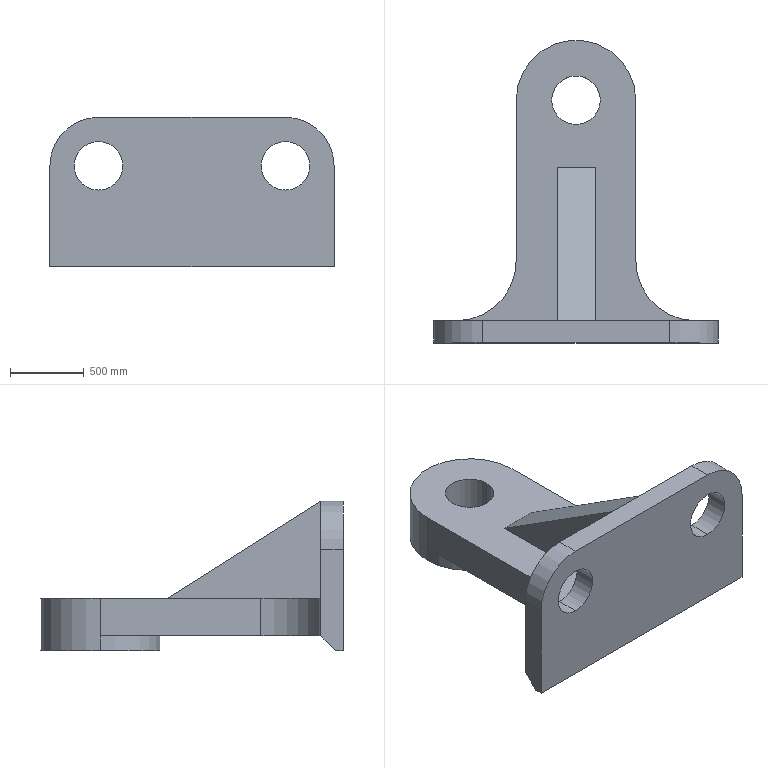Part | SolidWorks | features ICE 4, Chamfer 1, Extrusion 1, Fillet 1 | 1 solid | 28 faces | box 1930 x 2057 x 1016 mm | volume 760890020 mm3 | plane 16 | cylinder 12 | commonest cylinder face diameters 330.2 x6 812.8 x4 660.4 x2
STEP:
#1=CARTESIAN_POINT('',(6.5,65.,-6.));
#2=VERTEX_POINT('',#1);
#3=CARTESIAN_POINT('',(-6.5,65.,-6.));
#4=VERTEX_POINT('',#3);
#5=CARTESIAN_POINT('',(0.,65.,-6.));
#6=DIRECTION('',(0.,0.,-1.));
#7=DIRECTION('',(-1.,0.,0.));
#8=AXIS2_PLACEMENT_3D('',#5,#6,#7);
#9=CIRCLE('',#8,6.5);
#10=EDGE_CURVE('',#2,#4,#9,.T.);
#11=ORIENTED_EDGE('',*,*,#10,.F.);
#12=CARTESIAN_POINT('',(6.5,65.,-20.));
#13=VERTEX_POINT('',#12);
#14=CARTESIAN_POINT('',(6.5,65.,-6.));
#15=DIRECTION('',(0.,0.,-1.));
#16=VECTOR('',#15,39.37);
#17=LINE('',#14,#16);
#18=EDGE_CURVE('',#2,#13,#17,.T.);
#19=ORIENTED_EDGE('',*,*,#18,.T.);
#20=CARTESIAN_POINT('',(-6.5,65.,-20.));
#21=VERTEX_POINT('',#20);
#22=CARTESIAN_POINT('',(0.,65.,-20.));
#23=DIRECTION('',(0.,0.,-1.));
#24=DIRECTION('',(-1.,0.,0.));
#25=AXIS2_PLACEMENT_3D('',#22,#23,#24);
#26=CIRCLE('',#25,6.5);
#27=EDGE_CURVE('',#13,#21,#26,.T.);
#28=ORIENTED_EDGE('',*,*,#27,.T.);
#29=CARTESIAN_POINT('',(-6.5,65.,-6.));
#30=DIRECTION('',(0.,0.,-1.));
#31=VECTOR('',#30,39.37);
#32=LINE('',#29,#31);
#33=EDGE_CURVE('',#4,#21,#32,.T.);
#34=ORIENTED_EDGE('',*,*,#33,.F.);
#35=EDGE_LOOP('',(#11,#19,#28,#34));
#36=FACE_OUTER_BOUND('',#35,.T.);
#37=CARTESIAN_POINT('',(0.,65.,-6.));
#38=DIRECTION('',(0.,0.,-1.));
#39=DIRECTION('',(-1.,0.,0.));
#40=AXIS2_PLACEMENT_3D('',#37,#38,#39);
#41=CYLINDRICAL_SURFACE('',#40,6.5);
#42=ADVANCED_FACE('',(#36),#41,.F.);
#43=CARTESIAN_POINT('',(16.,65.,-6.));
#44=VERTEX_POINT('',#43);
#45=CARTESIAN_POINT('',(16.,65.,-16.));
#46=VERTEX_POINT('',#45);
#47=CARTESIAN_POINT('',(16.,65.,-6.));
#48=DIRECTION('',(0.,0.,-1.));
#49=VECTOR('',#48,39.37);
#50=LINE('',#47,#49);
#51=EDGE_CURVE('',#44,#46,#50,.T.);
#52=ORIENTED_EDGE('',*,*,#51,.T.);
#53=CARTESIAN_POINT('',(16.,65.,-20.));
#54=VERTEX_POINT('',#53);
#55=CARTESIAN_POINT('',(16.,65.,-6.));
#56=DIRECTION('',(0.,0.,-1.));
#57=VECTOR('',#56,39.37);
#58=LINE('',#55,#57);
#59=EDGE_CURVE('',#46,#54,#58,.T.);
#60=ORIENTED_EDGE('',*,*,#59,.T.);
#61=CARTESIAN_POINT('',(-16.,65.,-20.));
#62=VERTEX_POINT('',#61);
#63=CARTESIAN_POINT('',(0.,65.,-20.));
#64=DIRECTION('',(0.,0.,-1.));
#65=DIRECTION('',(-1.,0.,0.));
#66=AXIS2_PLACEMENT_3D('',#63,#64,#65);
#67=CIRCLE('',#66,16.);
#68=EDGE_CURVE('',#62,#54,#67,.T.);
#69=ORIENTED_EDGE('',*,*,#68,.F.);
#70=CARTESIAN_POINT('',(-16.,65.,-16.));
#71=VERTEX_POINT('',#70);
#72=CARTESIAN_POINT('',(-16.,65.,-6.));
#73=DIRECTION('',(0.,0.,-1.));
#74=VECTOR('',#73,39.37);
#75=LINE('',#72,#74);
#76=EDGE_CURVE('',#71,#62,#75,.T.);
#77=ORIENTED_EDGE('',*,*,#76,.F.);
#78=CARTESIAN_POINT('',(-16.,65.,-6.));
#79=VERTEX_POINT('',#78);
#80=CARTESIAN_POINT('',(-16.,65.,-6.));
#81=DIRECTION('',(0.,0.,-1.));
#82=VECTOR('',#81,39.37);
#83=LINE('',#80,#82);
#84=EDGE_CURVE('',#79,#71,#83,.T.);
#85=ORIENTED_EDGE('',*,*,#84,.F.);
#86=CARTESIAN_POINT('',(0.,65.,-6.));
#87=DIRECTION('',(0.,0.,-1.));
#88=DIRECTION('',(-1.,0.,0.));
#89=AXIS2_PLACEMENT_3D('',#86,#87,#88);
#90=CIRCLE('',#89,16.);
#91=EDGE_CURVE('',#79,#44,#90,.T.);
#92=ORIENTED_EDGE('',*,*,#91,.T.);
#93=EDGE_LOOP('',(#52,#60,#69,#77,#85,#92));
#94=FACE_OUTER_BOUND('',#93,.T.);
#95=CARTESIAN_POINT('',(0.,65.,-6.));
#96=DIRECTION('',(0.,0.,-1.));
#97=DIRECTION('',(-1.,0.,0.));
#98=AXIS2_PLACEMENT_3D('',#95,#96,#97);
#99=CYLINDRICAL_SURFACE('',#98,16.);
#100=ADVANCED_FACE('',(#94),#99,.T.);
#101=CARTESIAN_POINT('',(25.,6.,0.5));
#102=VERTEX_POINT('',#101);
#103=CARTESIAN_POINT('',(25.,6.,13.5));
#104=VERTEX_POINT('',#103);
#105=CARTESIAN_POINT('',(25.,6.,7.));
#106=DIRECTION('',(0.,1.,0.));
#107=DIRECTION('',(0.,0.,1.));
#108=AXIS2_PLACEMENT_3D('',#105,#106,#107);
#109=CIRCLE('',#108,6.5);
#110=EDGE_CURVE('',#102,#104,#109,.T.);
#111=ORIENTED_EDGE('',*,*,#110,.T.);
#112=CARTESIAN_POINT('',(25.,0.,13.5));
#113=VERTEX_POINT('',#112);
#114=CARTESIAN_POINT('',(25.,6.,13.5));
#115=DIRECTION('',(0.,-1.,0.));
#116=VECTOR('',#115,39.37);
#117=LINE('',#114,#116);
#118=EDGE_CURVE('',#104,#113,#117,.T.);
#119=ORIENTED_EDGE('',*,*,#118,.T.);
#120=CARTESIAN_POINT('',(25.,0.,0.5));
#121=VERTEX_POINT('',#120);
#122=CARTESIAN_POINT('',(25.,0.,7.));
#123=DIRECTION('',(0.,1.,0.));
#124=DIRECTION('',(0.,0.,1.));
#125=AXIS2_PLACEMENT_3D('',#122,#123,#124);
#126=CIRCLE('',#125,6.5);
#127=EDGE_CURVE('',#121,#113,#126,.T.);
#128=ORIENTED_EDGE('',*,*,#127,.F.);
#129=CARTESIAN_POINT('',(25.,6.,0.5));
#130=DIRECTION('',(0.,-1.,0.));
#131=VECTOR('',#130,39.37);
#132=LINE('',#129,#131);
#133=EDGE_CURVE('',#102,#121,#132,.T.);
#134=ORIENTED_EDGE('',*,*,#133,.F.);
#135=EDGE_LOOP('',(#111,#119,#128,#134));
#136=FACE_OUTER_BOUND('',#135,.T.);
#137=CARTESIAN_POINT('',(25.,6.,7.));
#138=DIRECTION('',(0.,-1.,0.));
#139=DIRECTION('',(0.,0.,-1.));
#140=AXIS2_PLACEMENT_3D('',#137,#138,#139);
#141=CYLINDRICAL_SURFACE('',#140,6.5);
#142=ADVANCED_FACE('',(#136),#141,.F.);
#143=CARTESIAN_POINT('',(-25.,6.,0.5));
#144=VERTEX_POINT('',#143);
#145=CARTESIAN_POINT('',(-25.,6.,13.5));
#146=VERTEX_POINT('',#145);
#147=CARTESIAN_POINT('',(-25.,6.,7.));
#148=DIRECTION('',(0.,1.,0.));
#149=DIRECTION('',(0.,0.,1.));
#150=AXIS2_PLACEMENT_3D('',#147,#148,#149);
#151=CIRCLE('',#150,6.5);
#152=EDGE_CURVE('',#144,#146,#151,.T.);
#153=ORIENTED_EDGE('',*,*,#152,.T.);
#154=CARTESIAN_POINT('',(-25.,0.,13.5));
#155=VERTEX_POINT('',#154);
#156=CARTESIAN_POINT('',(-25.,6.,13.5));
#157=DIRECTION('',(0.,-1.,0.));
#158=VECTOR('',#157,39.37);
#159=LINE('',#156,#158);
#160=EDGE_CURVE('',#146,#155,#159,.T.);
#161=ORIENTED_EDGE('',*,*,#160,.T.);
#162=CARTESIAN_POINT('',(-25.,0.,0.5));
#163=VERTEX_POINT('',#162);
#164=CARTESIAN_POINT('',(-25.,0.,7.));
#165=DIRECTION('',(0.,1.,0.));
#166=DIRECTION('',(0.,0.,1.));
#167=AXIS2_PLACEMENT_3D('',#164,#165,#166);
#168=CIRCLE('',#167,6.5);
#169=EDGE_CURVE('',#163,#155,#168,.T.);
#170=ORIENTED_EDGE('',*,*,#169,.F.);
#171=CARTESIAN_POINT('',(-25.,6.,0.5));
#172=DIRECTION('',(0.,-1.,0.));
#173=VECTOR('',#172,39.37);
#174=LINE('',#171,#173);
#175=EDGE_CURVE('',#144,#163,#174,.T.);
#176=ORIENTED_EDGE('',*,*,#175,.F.);
#177=EDGE_LOOP('',(#153,#161,#170,#176));
#178=FACE_OUTER_BOUND('',#177,.T.);
#179=CARTESIAN_POINT('',(-25.,6.,7.));
#180=DIRECTION('',(0.,-1.,0.));
#181=DIRECTION('',(0.,0.,-1.));
#182=AXIS2_PLACEMENT_3D('',#179,#180,#181);
#183=CYLINDRICAL_SURFACE('',#182,6.5);
#184=ADVANCED_FACE('',(#178),#183,.F.);
#185=ORIENTED_EDGE('',*,*,#110,.F.);
#186=CARTESIAN_POINT('',(25.,6.,7.));
#187=DIRECTION('',(0.,1.,0.));
#188=DIRECTION('',(0.,0.,1.));
#189=AXIS2_PLACEMENT_3D('',#186,#187,#188);
#190=CIRCLE('',#189,6.5);
#191=EDGE_CURVE('',#104,#102,#190,.T.);
#192=ORIENTED_EDGE('',*,*,#191,.F.);
#193=EDGE_LOOP('',(#185,#192));
#194=FACE_BOUND('',#193,.T.);
#195=CARTESIAN_POINT('',(38.,6.,7.));
#196=VERTEX_POINT('',#195);
#197=CARTESIAN_POINT('',(38.,6.,-16.));
#198=VERTEX_POINT('',#197);
#199=CARTESIAN_POINT('',(38.,6.,7.));
#200=DIRECTION('',(0.,0.,-1.));
#201=VECTOR('',#200,39.37);
#202=LINE('',#199,#201);
#203=EDGE_CURVE('',#196,#198,#202,.T.);
#204=ORIENTED_EDGE('',*,*,#203,.T.);
#205=CARTESIAN_POINT('',(32.,6.,-16.));
#206=VERTEX_POINT('',#205);
#207=CARTESIAN_POINT('',(-38.,6.,-16.));
#208=DIRECTION('',(-1.,0.,0.));
#209=VECTOR('',#208,39.37);
#210=LINE('',#207,#209);
#211=EDGE_CURVE('',#198,#206,#210,.T.);
#212=ORIENTED_EDGE('',*,*,#211,.T.);
#213=CARTESIAN_POINT('',(32.,6.,-6.));
#214=VERTEX_POINT('',#213);
#215=CARTESIAN_POINT('',(32.,6.,-6.));
#216=DIRECTION('',(0.,0.,1.));
#217=VECTOR('',#216,39.37);
#218=LINE('',#215,#217);
#219=EDGE_CURVE('',#206,#214,#218,.T.);
#220=ORIENTED_EDGE('',*,*,#219,.T.);
#221=CARTESIAN_POINT('',(5.262,6.,-6.));
#222=VERTEX_POINT('',#221);
#223=CARTESIAN_POINT('',(0.,6.,-6.));
#224=DIRECTION('',(1.,0.,0.));
#225=VECTOR('',#224,39.37);
#226=LINE('',#223,#225);
#227=EDGE_CURVE('',#222,#214,#226,.T.);
#228=ORIENTED_EDGE('',*,*,#227,.F.);
#229=CARTESIAN_POINT('',(5.262,6.,20.));
#230=VERTEX_POINT('',#229);
#231=CARTESIAN_POINT('',(5.262,6.,-6.));
#232=DIRECTION('',(0.,0.,-1.));
#233=VECTOR('',#232,39.37);
#234=LINE('',#231,#233);
#235=EDGE_CURVE('',#230,#222,#234,.T.);
#236=ORIENTED_EDGE('',*,*,#235,.F.);
#237=CARTESIAN_POINT('',(25.,6.,20.));
#238=VERTEX_POINT('',#237);
#239=CARTESIAN_POINT('',(25.,6.,20.));
#240=DIRECTION('',(1.,0.,0.));
#241=VECTOR('',#240,39.37);
#242=LINE('',#239,#241);
#243=EDGE_CURVE('',#230,#238,#242,.T.);
#244=ORIENTED_EDGE('',*,*,#243,.T.);
#245=CARTESIAN_POINT('',(25.,6.,7.));
#246=DIRECTION('',(0.,1.,0.));
#247=DIRECTION('',(0.,0.,1.));
#248=AXIS2_PLACEMENT_3D('',#245,#246,#247);
#249=CIRCLE('',#248,13.);
#250=EDGE_CURVE('',#238,#196,#249,.T.);
#251=ORIENTED_EDGE('',*,*,#250,.T.);
#252=EDGE_LOOP('',(#204,#212,#220,#228,#236,#244,#251));
#253=FACE_OUTER_BOUND('',#252,.T.);
#254=CARTESIAN_POINT('',(25.,6.,7.));
#255=DIRECTION('',(0.,1.,0.));
#256=DIRECTION('',(0.,0.,1.));
#257=AXIS2_PLACEMENT_3D('',#254,#255,#256);
#258=PLANE('',#257);
#259=ADVANCED_FACE('',(#194,#253),#258,.T.);
#260=ORIENTED_EDGE('',*,*,#152,.F.);
#261=CARTESIAN_POINT('',(-25.,6.,7.));
#262=DIRECTION('',(0.,1.,0.));
#263=DIRECTION('',(0.,0.,1.));
#264=AXIS2_PLACEMENT_3D('',#261,#262,#263);
#265=CIRCLE('',#264,6.5);
#266=EDGE_CURVE('',#146,#144,#265,.T.);
#267=ORIENTED_EDGE('',*,*,#266,.F.);
#268=EDGE_LOOP('',(#260,#267));
#269=FACE_BOUND('',#268,.T.);
#270=CARTESIAN_POINT('',(-32.,6.,-6.));
#271=VERTEX_POINT('',#270);
#272=CARTESIAN_POINT('',(-32.,6.,-16.));
#273=VERTEX_POINT('',#272);
#274=CARTESIAN_POINT('',(-32.,6.,7.));
#275=DIRECTION('',(0.,0.,-1.));
#276=VECTOR('',#275,39.37);
#277=LINE('',#274,#276);
#278=EDGE_CURVE('',#271,#273,#277,.T.);
#279=ORIENTED_EDGE('',*,*,#278,.T.);
#280=CARTESIAN_POINT('',(-38.,6.,-16.));
#281=VERTEX_POINT('',#280);
#282=CARTESIAN_POINT('',(-38.,6.,-16.));
#283=DIRECTION('',(-1.,0.,0.));
#284=VECTOR('',#283,39.37);
#285=LINE('',#282,#284);
#286=EDGE_CURVE('',#273,#281,#285,.T.);
#287=ORIENTED_EDGE('',*,*,#286,.T.);
#288=CARTESIAN_POINT('',(-38.,6.,7.));
#289=VERTEX_POINT('',#288);
#290=CARTESIAN_POINT('',(-38.,6.,7.));
#291=DIRECTION('',(0.,0.,1.));
#292=VECTOR('',#291,39.37);
#293=LINE('',#290,#292);
#294=EDGE_CURVE('',#281,#289,#293,.T.);
#295=ORIENTED_EDGE('',*,*,#294,.T.);
#296=CARTESIAN_POINT('',(-25.,6.,20.));
#297=VERTEX_POINT('',#296);
#298=CARTESIAN_POINT('',(-25.,6.,7.));
#299=DIRECTION('',(0.,1.,0.));
#300=DIRECTION('',(0.,0.,-1.));
#301=AXIS2_PLACEMENT_3D('',#298,#299,#300);
#302=CIRCLE('',#301,13.);
#303=EDGE_CURVE('',#289,#297,#302,.T.);
#304=ORIENTED_EDGE('',*,*,#303,.T.);
#305=CARTESIAN_POINT('',(-5.,6.,20.));
#306=VERTEX_POINT('',#305);
#307=CARTESIAN_POINT('',(25.,6.,20.));
#308=DIRECTION('',(1.,0.,0.));
#309=VECTOR('',#308,39.37);
#310=LINE('',#307,#309);
#311=EDGE_CURVE('',#297,#306,#310,.T.);
#312=ORIENTED_EDGE('',*,*,#311,.T.);
#313=CARTESIAN_POINT('',(-5.,6.,-6.));
#314=VERTEX_POINT('',#313);
#315=CARTESIAN_POINT('',(-5.,6.,-6.));
#316=DIRECTION('',(0.,0.,1.));
#317=VECTOR('',#316,39.37);
#318=LINE('',#315,#317);
#319=EDGE_CURVE('',#314,#306,#318,.T.);
#320=ORIENTED_EDGE('',*,*,#319,.F.);
#321=CARTESIAN_POINT('',(0.,6.,-6.));
#322=DIRECTION('',(1.,0.,0.));
#323=VECTOR('',#322,39.37);
#324=LINE('',#321,#323);
#325=EDGE_CURVE('',#271,#314,#324,.T.);
#326=ORIENTED_EDGE('',*,*,#325,.F.);
#327=EDGE_LOOP('',(#279,#287,#295,#304,#312,#320,#326));
#328=FACE_OUTER_BOUND('',#327,.T.);
#329=CARTESIAN_POINT('',(25.,6.,7.));
#330=DIRECTION('',(0.,1.,0.));
#331=DIRECTION('',(0.,0.,1.));
#332=AXIS2_PLACEMENT_3D('',#329,#330,#331);
#333=PLANE('',#332);
#334=ADVANCED_FACE('',(#269,#328),#333,.T.);
#335=CARTESIAN_POINT('',(-5.,47.,-6.));
#336=VERTEX_POINT('',#335);
#337=CARTESIAN_POINT('',(-5.,47.,-6.));
#338=DIRECTION('',(0.,-1.,0.));
#339=VECTOR('',#338,39.37);
#340=LINE('',#337,#339);
#341=EDGE_CURVE('',#336,#314,#340,.T.);
#342=ORIENTED_EDGE('',*,*,#341,.F.);
#343=CARTESIAN_POINT('',(5.262,47.,-6.));
#344=VERTEX_POINT('',#343);
#345=CARTESIAN_POINT('',(-5.,47.,-6.));
#346=DIRECTION('',(-1.,0.,0.));
#347=VECTOR('',#346,39.37);
#348=LINE('',#345,#347);
#349=EDGE_CURVE('',#344,#336,#348,.T.);
#350=ORIENTED_EDGE('',*,*,#349,.F.);
#351=CARTESIAN_POINT('',(5.262,47.,-6.));
#352=DIRECTION('',(0.,-1.,0.));
#353=VECTOR('',#352,39.37);
#354=LINE('',#351,#353);
#355=EDGE_CURVE('',#344,#222,#354,.T.);
#356=ORIENTED_EDGE('',*,*,#355,.T.);
#357=ORIENTED_EDGE('',*,*,#227,.T.);
#358=CARTESIAN_POINT('',(16.,22.,-6.));
#359=VERTEX_POINT('',#358);
#360=CARTESIAN_POINT('',(32.,22.,-6.));
#361=DIRECTION('',(0.,0.,-1.));
#362=DIRECTION('',(-1.,0.,0.));
#363=AXIS2_PLACEMENT_3D('',#360,#361,#362);
#364=CIRCLE('',#363,16.);
#365=EDGE_CURVE('',#214,#359,#364,.T.);
#366=ORIENTED_EDGE('',*,*,#365,.T.);
#367=CARTESIAN_POINT('',(16.,0.,-6.));
#368=DIRECTION('',(0.,-1.,0.));
#369=VECTOR('',#368,39.37);
#370=LINE('',#367,#369);
#371=EDGE_CURVE('',#44,#359,#370,.T.);
#372=ORIENTED_EDGE('',*,*,#371,.F.);
#373=ORIENTED_EDGE('',*,*,#91,.F.);
#374=CARTESIAN_POINT('',(-16.,22.,-6.));
#375=VERTEX_POINT('',#374);
#376=CARTESIAN_POINT('',(-16.,0.,-6.));
#377=DIRECTION('',(0.,-1.,0.));
#378=VECTOR('',#377,39.37);
#379=LINE('',#376,#378);
#380=EDGE_CURVE('',#79,#375,#379,.T.);
#381=ORIENTED_EDGE('',*,*,#380,.T.);
#382=CARTESIAN_POINT('',(-32.,22.,-6.));
#383=DIRECTION('',(0.,0.,-1.));
#384=DIRECTION('',(-1.,0.,0.));
#385=AXIS2_PLACEMENT_3D('',#382,#383,#384);
#386=CIRCLE('',#385,16.);
#387=EDGE_CURVE('',#375,#271,#386,.T.);
#388=ORIENTED_EDGE('',*,*,#387,.T.);
#389=ORIENTED_EDGE('',*,*,#325,.T.);
#390=EDGE_LOOP('',(#342,#350,#356,#357,#366,#372,#373,#381,#388,#389));
#391=FACE_OUTER_BOUND('',#390,.T.);
#392=CARTESIAN_POINT('',(0.,65.,-6.));
#393=DIRECTION('',(0.,0.,-1.));
#394=DIRECTION('',(-1.,0.,0.));
#395=AXIS2_PLACEMENT_3D('',#392,#393,#394);
#396=CIRCLE('',#395,6.5);
#397=EDGE_CURVE('',#4,#2,#396,.T.);
#398=ORIENTED_EDGE('',*,*,#397,.T.);
#399=ORIENTED_EDGE('',*,*,#10,.T.);
#400=EDGE_LOOP('',(#398,#399));
#401=FACE_BOUND('',#400,.T.);
#402=CARTESIAN_POINT('',(0.,0.,-6.));
#403=DIRECTION('',(0.,0.,-1.));
#404=DIRECTION('',(-1.,0.,0.));
#405=AXIS2_PLACEMENT_3D('',#402,#403,#404);
#406=PLANE('',#405);
#407=ADVANCED_FACE('',(#391,#401),#406,.F.);
#408=CARTESIAN_POINT('',(-16.,22.,-16.));
#409=VERTEX_POINT('',#408);
#410=CARTESIAN_POINT('',(-16.,0.,-16.));
#411=DIRECTION('',(0.,-1.,0.));
#412=VECTOR('',#411,39.37);
#413=LINE('',#410,#412);
#414=EDGE_CURVE('',#71,#409,#413,.T.);
#415=ORIENTED_EDGE('',*,*,#414,.F.);
#416=CARTESIAN_POINT('',(0.,65.,-16.));
#417=DIRECTION('',(0.,0.,1.));
#418=DIRECTION('',(-1.,0.,0.));
#419=AXIS2_PLACEMENT_3D('',#416,#417,#418);
#420=CIRCLE('',#419,16.);
#421=EDGE_CURVE('',#71,#46,#420,.T.);
#422=ORIENTED_EDGE('',*,*,#421,.T.);
#423=CARTESIAN_POINT('',(16.,22.,-16.));
#424=VERTEX_POINT('',#423);
#425=CARTESIAN_POINT('',(16.,0.,-16.));
#426=DIRECTION('',(0.,-1.,0.));
#427=VECTOR('',#426,39.37);
#428=LINE('',#425,#427);
#429=EDGE_CURVE('',#46,#424,#428,.T.);
#430=ORIENTED_EDGE('',*,*,#429,.T.);
#431=CARTESIAN_POINT('',(32.,22.,-16.));
#432=DIRECTION('',(0.,0.,1.));
#433=DIRECTION('',(-1.,0.,0.));
#434=AXIS2_PLACEMENT_3D('',#431,#432,#433);
#435=CIRCLE('',#434,16.);
#436=EDGE_CURVE('',#424,#206,#435,.T.);
#437=ORIENTED_EDGE('',*,*,#436,.T.);
#438=CARTESIAN_POINT('',(0.,6.,-16.));
#439=DIRECTION('',(1.,0.,0.));
#440=VECTOR('',#439,39.37);
#441=LINE('',#438,#440);
#442=EDGE_CURVE('',#273,#206,#441,.T.);
#443=ORIENTED_EDGE('',*,*,#442,.F.);
#444=CARTESIAN_POINT('',(-32.,22.,-16.));
#445=DIRECTION('',(0.,0.,1.));
#446=DIRECTION('',(-1.,0.,0.));
#447=AXIS2_PLACEMENT_3D('',#444,#445,#446);
#448=CIRCLE('',#447,16.);
#449=EDGE_CURVE('',#273,#409,#448,.T.);
#450=ORIENTED_EDGE('',*,*,#449,.T.);
#451=EDGE_LOOP('',(#415,#422,#430,#437,#443,#450));
#452=FACE_OUTER_BOUND('',#451,.T.);
#453=CARTESIAN_POINT('',(0.,0.,-16.));
#454=DIRECTION('',(0.,0.,-1.));
#455=DIRECTION('',(-1.,0.,0.));
#456=AXIS2_PLACEMENT_3D('',#453,#454,#455);
#457=PLANE('',#456);
#458=ADVANCED_FACE('',(#452),#457,.T.);
#459=CARTESIAN_POINT('',(-38.,0.,-20.));
#460=VERTEX_POINT('',#459);
#461=CARTESIAN_POINT('',(-38.,0.,7.));
#462=VERTEX_POINT('',#461);
#463=CARTESIAN_POINT('',(-38.,0.,7.));
#464=DIRECTION('',(0.,0.,1.));
#465=VECTOR('',#464,39.37);
#466=LINE('',#463,#465);
#467=EDGE_CURVE('',#460,#462,#466,.T.);
#468=ORIENTED_EDGE('',*,*,#467,.F.);
#469=CARTESIAN_POINT('',(38.,0.,-20.));
#470=VERTEX_POINT('',#469);
#471=CARTESIAN_POINT('',(38.,0.,-20.));
#472=DIRECTION('',(-1.,0.,0.));
#473=VECTOR('',#472,39.37);
#474=LINE('',#471,#473);
#475=EDGE_CURVE('',#470,#460,#474,.T.);
#476=ORIENTED_EDGE('',*,*,#475,.F.);
#477=CARTESIAN_POINT('',(38.,0.,7.));
#478=VERTEX_POINT('',#477);
#479=CARTESIAN_POINT('',(38.,0.,7.));
#480=DIRECTION('',(0.,0.,-1.));
#481=VECTOR('',#480,39.37);
#482=LINE('',#479,#481);
#483=EDGE_CURVE('',#478,#470,#482,.T.);
#484=ORIENTED_EDGE('',*,*,#483,.F.);
#485=CARTESIAN_POINT('',(25.,0.,20.));
#486=VERTEX_POINT('',#485);
#487=CARTESIAN_POINT('',(25.,0.,7.));
#488=DIRECTION('',(0.,1.,0.));
#489=DIRECTION('',(0.,0.,1.));
#490=AXIS2_PLACEMENT_3D('',#487,#488,#489);
#491=CIRCLE('',#490,13.);
#492=EDGE_CURVE('',#486,#478,#491,.T.);
#493=ORIENTED_EDGE('',*,*,#492,.F.);
#494=CARTESIAN_POINT('',(-25.,0.,20.));
#495=VERTEX_POINT('',#494);
#496=CARTESIAN_POINT('',(25.,0.,20.));
#497=DIRECTION('',(1.,0.,0.));
#498=VECTOR('',#497,39.37);
#499=LINE('',#496,#498);
#500=EDGE_CURVE('',#495,#486,#499,.T.);
#501=ORIENTED_EDGE('',*,*,#500,.F.);
#502=CARTESIAN_POINT('',(-25.,0.,7.));
#503=DIRECTION('',(0.,1.,0.));
#504=DIRECTION('',(0.,0.,-1.));
#505=AXIS2_PLACEMENT_3D('',#502,#503,#504);
#506=CIRCLE('',#505,13.);
#507=EDGE_CURVE('',#462,#495,#506,.T.);
#508=ORIENTED_EDGE('',*,*,#507,.F.);
#509=EDGE_LOOP('',(#468,#476,#484,#493,#501,#508));
#510=FACE_OUTER_BOUND('',#509,.T.);
#511=ORIENTED_EDGE('',*,*,#169,.T.);
#512=CARTESIAN_POINT('',(-25.,0.,7.));
#513=DIRECTION('',(0.,1.,0.));
#514=DIRECTION('',(0.,0.,1.));
#515=AXIS2_PLACEMENT_3D('',#512,#513,#514);
#516=CIRCLE('',#515,6.5);
#517=EDGE_CURVE('',#155,#163,#516,.T.);
#518=ORIENTED_EDGE('',*,*,#517,.T.);
#519=EDGE_LOOP('',(#511,#518));
#520=FACE_BOUND('',#519,.T.);
#521=ORIENTED_EDGE('',*,*,#127,.T.);
#522=CARTESIAN_POINT('',(25.,0.,7.));
#523=DIRECTION('',(0.,1.,0.));
#524=DIRECTION('',(0.,0.,1.));
#525=AXIS2_PLACEMENT_3D('',#522,#523,#524);
#526=CIRCLE('',#525,6.5);
#527=EDGE_CURVE('',#113,#121,#526,.T.);
#528=ORIENTED_EDGE('',*,*,#527,.T.);
#529=EDGE_LOOP('',(#521,#528));
#530=FACE_BOUND('',#529,.T.);
#531=CARTESIAN_POINT('',(25.,0.,7.));
#532=DIRECTION('',(0.,1.,0.));
#533=DIRECTION('',(0.,0.,1.));
#534=AXIS2_PLACEMENT_3D('',#531,#532,#533);
#535=PLANE('',#534);
#536=ADVANCED_FACE('',(#510,#520,#530),#535,.F.);
#537=ORIENTED_EDGE('',*,*,#294,.F.);
#538=CARTESIAN_POINT('',(-38.,2.,-20.));
#539=VERTEX_POINT('',#538);
#540=CARTESIAN_POINT('',(-38.,6.,-16.));
#541=DIRECTION('',(0.,-0.7071,-0.7071));
#542=VECTOR('',#541,39.37);
#543=LINE('',#540,#542);
#544=EDGE_CURVE('',#281,#539,#543,.T.);
#545=ORIENTED_EDGE('',*,*,#544,.T.);
#546=CARTESIAN_POINT('',(-38.,6.,-20.));
#547=DIRECTION('',(0.,-1.,0.));
#548=VECTOR('',#547,39.37);
#549=LINE('',#546,#548);
#550=EDGE_CURVE('',#539,#460,#549,.T.);
#551=ORIENTED_EDGE('',*,*,#550,.T.);
#552=ORIENTED_EDGE('',*,*,#467,.T.);
#553=CARTESIAN_POINT('',(-38.,6.,7.));
#554=DIRECTION('',(0.,-1.,0.));
#555=VECTOR('',#554,39.37);
#556=LINE('',#553,#555);
#557=EDGE_CURVE('',#289,#462,#556,.T.);
#558=ORIENTED_EDGE('',*,*,#557,.F.);
#559=EDGE_LOOP('',(#537,#545,#551,#552,#558));
#560=FACE_OUTER_BOUND('',#559,.T.);
#561=CARTESIAN_POINT('',(-38.,6.,7.));
#562=DIRECTION('',(1.,0.,0.));
#563=DIRECTION('',(0.,0.,-1.));
#564=AXIS2_PLACEMENT_3D('',#561,#562,#563);
#565=PLANE('',#564);
#566=ADVANCED_FACE('',(#560),#565,.F.);
#567=ORIENTED_EDGE('',*,*,#507,.T.);
#568=CARTESIAN_POINT('',(-25.,6.,20.));
#569=DIRECTION('',(0.,-1.,0.));
#570=VECTOR('',#569,39.37);
#571=LINE('',#568,#570);
#572=EDGE_CURVE('',#297,#495,#571,.T.);
#573=ORIENTED_EDGE('',*,*,#572,.F.);
#574=ORIENTED_EDGE('',*,*,#303,.F.);
#575=ORIENTED_EDGE('',*,*,#557,.T.);
#576=EDGE_LOOP('',(#567,#573,#574,#575));
#577=FACE_OUTER_BOUND('',#576,.T.);
#578=CARTESIAN_POINT('',(-25.,6.,7.));
#579=DIRECTION('',(0.,-1.,0.));
#580=DIRECTION('',(0.,0.,-1.));
#581=AXIS2_PLACEMENT_3D('',#578,#579,#580);
#582=CYLINDRICAL_SURFACE('',#581,13.);
#583=ADVANCED_FACE('',(#577),#582,.T.);
#584=ORIENTED_EDGE('',*,*,#243,.F.);
#585=CARTESIAN_POINT('',(-38.,6.,20.));
#586=DIRECTION('',(1.,0.,0.));
#587=VECTOR('',#586,39.37);
#588=LINE('',#585,#587);
#589=EDGE_CURVE('',#306,#230,#588,.T.);
#590=ORIENTED_EDGE('',*,*,#589,.F.);
#591=ORIENTED_EDGE('',*,*,#311,.F.);
#592=ORIENTED_EDGE('',*,*,#572,.T.);
#593=ORIENTED_EDGE('',*,*,#500,.T.);
#594=CARTESIAN_POINT('',(25.,6.,20.));
#595=DIRECTION('',(0.,-1.,0.));
#596=VECTOR('',#595,39.37);
#597=LINE('',#594,#596);
#598=EDGE_CURVE('',#238,#486,#597,.T.);
#599=ORIENTED_EDGE('',*,*,#598,.F.);
#600=EDGE_LOOP('',(#584,#590,#591,#592,#593,#599));
#601=FACE_OUTER_BOUND('',#600,.T.);
#602=CARTESIAN_POINT('',(25.,6.,20.));
#603=DIRECTION('',(0.,0.,-1.));
#604=DIRECTION('',(-1.,0.,0.));
#605=AXIS2_PLACEMENT_3D('',#602,#603,#604);
#606=PLANE('',#605);
#607=ADVANCED_FACE('',(#601),#606,.F.);
#608=ORIENTED_EDGE('',*,*,#492,.T.);
#609=CARTESIAN_POINT('',(38.,6.,7.));
#610=DIRECTION('',(0.,-1.,0.));
#611=VECTOR('',#610,39.37);
#612=LINE('',#609,#611);
#613=EDGE_CURVE('',#196,#478,#612,.T.);
#614=ORIENTED_EDGE('',*,*,#613,.F.);
#615=ORIENTED_EDGE('',*,*,#250,.F.);
#616=ORIENTED_EDGE('',*,*,#598,.T.);
#617=EDGE_LOOP('',(#608,#614,#615,#616));
#618=FACE_OUTER_BOUND('',#617,.T.);
#619=CARTESIAN_POINT('',(25.,6.,7.));
#620=DIRECTION('',(0.,-1.,0.));
#621=DIRECTION('',(0.,0.,-1.));
#622=AXIS2_PLACEMENT_3D('',#619,#620,#621);
#623=CYLINDRICAL_SURFACE('',#622,13.);
#624=ADVANCED_FACE('',(#618),#623,.T.);
#625=CARTESIAN_POINT('',(38.,2.,-20.));
#626=VERTEX_POINT('',#625);
#627=CARTESIAN_POINT('',(38.,6.,-20.));
#628=DIRECTION('',(0.,-1.,0.));
#629=VECTOR('',#628,39.37);
#630=LINE('',#627,#629);
#631=EDGE_CURVE('',#626,#470,#630,.T.);
#632=ORIENTED_EDGE('',*,*,#631,.F.);
#633=CARTESIAN_POINT('',(38.,6.,-16.));
#634=DIRECTION('',(0.,0.7071,0.7071));
#635=VECTOR('',#634,39.37);
#636=LINE('',#633,#635);
#637=EDGE_CURVE('',#626,#198,#636,.T.);
#638=ORIENTED_EDGE('',*,*,#637,.T.);
#639=ORIENTED_EDGE('',*,*,#203,.F.);
#640=ORIENTED_EDGE('',*,*,#613,.T.);
#641=ORIENTED_EDGE('',*,*,#483,.T.);
#642=EDGE_LOOP('',(#632,#638,#639,#640,#641));
#643=FACE_OUTER_BOUND('',#642,.T.);
#644=CARTESIAN_POINT('',(38.,6.,7.));
#645=DIRECTION('',(-1.,0.,0.));
#646=DIRECTION('',(0.,0.,1.));
#647=AXIS2_PLACEMENT_3D('',#644,#645,#646);
#648=PLANE('',#647);
#649=ADVANCED_FACE('',(#643),#648,.F.);
#650=ORIENTED_EDGE('',*,*,#550,.F.);
#651=CARTESIAN_POINT('',(38.,2.,-20.));
#652=DIRECTION('',(1.,0.,0.));
#653=VECTOR('',#652,39.37);
#654=LINE('',#651,#653);
#655=EDGE_CURVE('',#539,#626,#654,.T.);
#656=ORIENTED_EDGE('',*,*,#655,.T.);
#657=ORIENTED_EDGE('',*,*,#631,.T.);
#658=ORIENTED_EDGE('',*,*,#475,.T.);
#659=EDGE_LOOP('',(#650,#656,#657,#658));
#660=FACE_OUTER_BOUND('',#659,.T.);
#661=CARTESIAN_POINT('',(38.,6.,-20.));
#662=DIRECTION('',(0.,0.,1.));
#663=DIRECTION('',(1.,0.,0.));
#664=AXIS2_PLACEMENT_3D('',#661,#662,#663);
#665=PLANE('',#664);
#666=ADVANCED_FACE('',(#660),#665,.F.);
#667=ORIENTED_EDGE('',*,*,#160,.F.);
#668=ORIENTED_EDGE('',*,*,#266,.T.);
#669=ORIENTED_EDGE('',*,*,#175,.T.);
#670=ORIENTED_EDGE('',*,*,#517,.F.);
#671=EDGE_LOOP('',(#667,#668,#669,#670));
#672=FACE_OUTER_BOUND('',#671,.T.);
#673=CARTESIAN_POINT('',(-25.,6.,7.));
#674=DIRECTION('',(0.,-1.,0.));
#675=DIRECTION('',(0.,0.,-1.));
#676=AXIS2_PLACEMENT_3D('',#673,#674,#675);
#677=CYLINDRICAL_SURFACE('',#676,6.5);
#678=ADVANCED_FACE('',(#672),#677,.F.);
#679=ORIENTED_EDGE('',*,*,#118,.F.);
#680=ORIENTED_EDGE('',*,*,#191,.T.);
#681=ORIENTED_EDGE('',*,*,#133,.T.);
#682=ORIENTED_EDGE('',*,*,#527,.F.);
#683=EDGE_LOOP('',(#679,#680,#681,#682));
#684=FACE_OUTER_BOUND('',#683,.T.);
#685=CARTESIAN_POINT('',(25.,6.,7.));
#686=DIRECTION('',(0.,-1.,0.));
#687=DIRECTION('',(0.,0.,-1.));
#688=AXIS2_PLACEMENT_3D('',#685,#686,#687);
#689=CYLINDRICAL_SURFACE('',#688,6.5);
#690=ADVANCED_FACE('',(#684),#689,.F.);
#691=ORIENTED_EDGE('',*,*,#414,.T.);
#692=CARTESIAN_POINT('',(-16.,22.,-6.));
#693=DIRECTION('',(0.,0.,1.));
#694=VECTOR('',#693,39.37);
#695=LINE('',#692,#694);
#696=EDGE_CURVE('',#409,#375,#695,.T.);
#697=ORIENTED_EDGE('',*,*,#696,.T.);
#698=ORIENTED_EDGE('',*,*,#380,.F.);
#699=ORIENTED_EDGE('',*,*,#84,.T.);
#700=EDGE_LOOP('',(#691,#697,#698,#699));
#701=FACE_OUTER_BOUND('',#700,.T.);
#702=CARTESIAN_POINT('',(-16.,0.,-6.));
#703=DIRECTION('',(1.,0.,0.));
#704=DIRECTION('',(0.,1.,0.));
#705=AXIS2_PLACEMENT_3D('',#702,#703,#704);
#706=PLANE('',#705);
#707=ADVANCED_FACE('',(#701),#706,.F.);
#708=ORIENTED_EDGE('',*,*,#371,.T.);
#709=CARTESIAN_POINT('',(16.,22.,-16.));
#710=DIRECTION('',(0.,0.,-1.));
#711=VECTOR('',#710,39.37);
#712=LINE('',#709,#711);
#713=EDGE_CURVE('',#359,#424,#712,.T.);
#714=ORIENTED_EDGE('',*,*,#713,.T.);
#715=ORIENTED_EDGE('',*,*,#429,.F.);
#716=ORIENTED_EDGE('',*,*,#51,.F.);
#717=EDGE_LOOP('',(#708,#714,#715,#716));
#718=FACE_OUTER_BOUND('',#717,.T.);
#719=CARTESIAN_POINT('',(16.,0.,-6.));
#720=DIRECTION('',(1.,0.,0.));
#721=DIRECTION('',(0.,1.,0.));
#722=AXIS2_PLACEMENT_3D('',#719,#720,#721);
#723=PLANE('',#722);
#724=ADVANCED_FACE('',(#718),#723,.T.);
#725=ORIENTED_EDGE('',*,*,#59,.F.);
#726=ORIENTED_EDGE('',*,*,#421,.F.);
#727=ORIENTED_EDGE('',*,*,#76,.T.);
#728=CARTESIAN_POINT('',(0.,65.,-20.));
#729=DIRECTION('',(0.,0.,-1.));
#730=DIRECTION('',(-1.,0.,0.));
#731=AXIS2_PLACEMENT_3D('',#728,#729,#730);
#732=CIRCLE('',#731,16.);
#733=EDGE_CURVE('',#54,#62,#732,.T.);
#734=ORIENTED_EDGE('',*,*,#733,.F.);
#735=EDGE_LOOP('',(#725,#726,#727,#734));
#736=FACE_OUTER_BOUND('',#735,.T.);
#737=CARTESIAN_POINT('',(0.,65.,-6.));
#738=DIRECTION('',(0.,0.,-1.));
#739=DIRECTION('',(-1.,0.,0.));
#740=AXIS2_PLACEMENT_3D('',#737,#738,#739);
#741=CYLINDRICAL_SURFACE('',#740,16.);
#742=ADVANCED_FACE('',(#736),#741,.T.);
#743=ORIENTED_EDGE('',*,*,#18,.F.);
#744=ORIENTED_EDGE('',*,*,#397,.F.);
#745=ORIENTED_EDGE('',*,*,#33,.T.);
#746=CARTESIAN_POINT('',(0.,65.,-20.));
#747=DIRECTION('',(0.,0.,-1.));
#748=DIRECTION('',(-1.,0.,0.));
#749=AXIS2_PLACEMENT_3D('',#746,#747,#748);
#750=CIRCLE('',#749,6.5);
#751=EDGE_CURVE('',#21,#13,#750,.T.);
#752=ORIENTED_EDGE('',*,*,#751,.T.);
#753=EDGE_LOOP('',(#743,#744,#745,#752));
#754=FACE_OUTER_BOUND('',#753,.T.);
#755=CARTESIAN_POINT('',(0.,65.,-6.));
#756=DIRECTION('',(0.,0.,-1.));
#757=DIRECTION('',(-1.,0.,0.));
#758=AXIS2_PLACEMENT_3D('',#755,#756,#757);
#759=CYLINDRICAL_SURFACE('',#758,6.5);
#760=ADVANCED_FACE('',(#754),#759,.F.);
#761=ORIENTED_EDGE('',*,*,#751,.F.);
#762=ORIENTED_EDGE('',*,*,#27,.F.);
#763=EDGE_LOOP('',(#761,#762));
#764=FACE_BOUND('',#763,.T.);
#765=ORIENTED_EDGE('',*,*,#68,.T.);
#766=ORIENTED_EDGE('',*,*,#733,.T.);
#767=EDGE_LOOP('',(#765,#766));
#768=FACE_OUTER_BOUND('',#767,.T.);
#769=CARTESIAN_POINT('',(0.,0.,-20.));
#770=DIRECTION('',(0.,0.,-1.));
#771=DIRECTION('',(-1.,0.,0.));
#772=AXIS2_PLACEMENT_3D('',#769,#770,#771);
#773=PLANE('',#772);
#774=ADVANCED_FACE('',(#764,#768),#773,.T.);
#775=ORIENTED_EDGE('',*,*,#387,.F.);
#776=ORIENTED_EDGE('',*,*,#696,.F.);
#777=ORIENTED_EDGE('',*,*,#449,.F.);
#778=ORIENTED_EDGE('',*,*,#278,.F.);
#779=EDGE_LOOP('',(#775,#776,#777,#778));
#780=FACE_OUTER_BOUND('',#779,.T.);
#781=CARTESIAN_POINT('',(-32.,22.,7.));
#782=DIRECTION('',(0.,0.,-1.));
#783=DIRECTION('',(-1.,0.,0.));
#784=AXIS2_PLACEMENT_3D('',#781,#782,#783);
#785=CYLINDRICAL_SURFACE('',#784,16.);
#786=ADVANCED_FACE('',(#780),#785,.F.);
#787=ORIENTED_EDGE('',*,*,#365,.F.);
#788=ORIENTED_EDGE('',*,*,#219,.F.);
#789=ORIENTED_EDGE('',*,*,#436,.F.);
#790=ORIENTED_EDGE('',*,*,#713,.F.);
#791=EDGE_LOOP('',(#787,#788,#789,#790));
#792=FACE_OUTER_BOUND('',#791,.T.);
#793=CARTESIAN_POINT('',(32.,22.,-6.));
#794=DIRECTION('',(0.,0.,1.));
#795=DIRECTION('',(1.,0.,0.));
#796=AXIS2_PLACEMENT_3D('',#793,#794,#795);
#797=CYLINDRICAL_SURFACE('',#796,16.);
#798=ADVANCED_FACE('',(#792),#797,.F.);
#799=ORIENTED_EDGE('',*,*,#319,.T.);
#800=CARTESIAN_POINT('',(-5.,47.,-6.));
#801=DIRECTION('',(0.,0.8445,-0.5355));
#802=VECTOR('',#801,39.37);
#803=LINE('',#800,#802);
#804=EDGE_CURVE('',#306,#336,#803,.T.);
#805=ORIENTED_EDGE('',*,*,#804,.T.);
#806=ORIENTED_EDGE('',*,*,#341,.T.);
#807=EDGE_LOOP('',(#799,#805,#806));
#808=FACE_OUTER_BOUND('',#807,.T.);
#809=CARTESIAN_POINT('',(-5.,47.,-6.));
#810=DIRECTION('',(1.,0.,0.));
#811=DIRECTION('',(0.,0.,-1.));
#812=AXIS2_PLACEMENT_3D('',#809,#810,#811);
#813=PLANE('',#812);
#814=ADVANCED_FACE('',(#808),#813,.F.);
#815=ORIENTED_EDGE('',*,*,#355,.F.);
#816=CARTESIAN_POINT('',(5.262,47.,-6.));
#817=DIRECTION('',(0.,0.8445,-0.5355));
#818=VECTOR('',#817,39.37);
#819=LINE('',#816,#818);
#820=EDGE_CURVE('',#230,#344,#819,.T.);
#821=ORIENTED_EDGE('',*,*,#820,.F.);
#822=ORIENTED_EDGE('',*,*,#235,.T.);
#823=EDGE_LOOP('',(#815,#821,#822));
#824=FACE_OUTER_BOUND('',#823,.T.);
#825=CARTESIAN_POINT('',(5.262,47.,-6.));
#826=DIRECTION('',(-1.,0.,0.));
#827=DIRECTION('',(0.,0.,1.));
#828=AXIS2_PLACEMENT_3D('',#825,#826,#827);
#829=PLANE('',#828);
#830=ADVANCED_FACE('',(#824),#829,.F.);
#831=ORIENTED_EDGE('',*,*,#589,.T.);
#832=ORIENTED_EDGE('',*,*,#820,.T.);
#833=ORIENTED_EDGE('',*,*,#349,.T.);
#834=ORIENTED_EDGE('',*,*,#804,.F.);
#835=EDGE_LOOP('',(#831,#832,#833,#834));
#836=FACE_OUTER_BOUND('',#835,.T.);
#837=CARTESIAN_POINT('',(-38.,47.,-6.));
#838=DIRECTION('',(0.,-0.5355,-0.8445));
#839=DIRECTION('',(0.,0.8445,-0.5355));
#840=AXIS2_PLACEMENT_3D('',#837,#838,#839);
#841=PLANE('',#840);
#842=ADVANCED_FACE('',(#836),#841,.F.);
#843=ORIENTED_EDGE('',*,*,#637,.F.);
#844=ORIENTED_EDGE('',*,*,#655,.F.);
#845=ORIENTED_EDGE('',*,*,#544,.F.);
#846=ORIENTED_EDGE('',*,*,#286,.F.);
#847=ORIENTED_EDGE('',*,*,#442,.T.);
#848=ORIENTED_EDGE('',*,*,#211,.F.);
#849=EDGE_LOOP('',(#843,#844,#845,#846,#847,#848));
#850=FACE_OUTER_BOUND('',#849,.T.);
#851=CARTESIAN_POINT('',(25.,6.,-16.));
#852=DIRECTION('',(0.,0.7071,-0.7071));
#853=DIRECTION('',(1.,0.,0.));
#854=AXIS2_PLACEMENT_3D('',#851,#852,#853);
#855=PLANE('',#854);
#856=ADVANCED_FACE('',(#850),#855,.T.);
#857=CLOSED_SHELL('',(#42,#100,#142,#184,#259,#334,#407,#458,#536,#566,#583,#607,#624,#649,#666,#678,#690,#707,#724,#742,#760,#774,#786,#798,#814,#830,#842,#856));
#858=MANIFOLD_SOLID_BREP('',#857);
#859=CARTESIAN_POINT('',(0.,0.,0.));
#860=DIRECTION('',(0.,0.,1.));
#861=DIRECTION('',(1.,0.,0.));
#862=AXIS2_PLACEMENT_3D('',#859,#860,#861);
#863=(LENGTH_UNIT()NAMED_UNIT(*)SI_UNIT($,.METRE.));
#864=LENGTH_MEASURE_WITH_UNIT(LENGTH_MEASURE(0.0254),#863);
#865=DIMENSIONAL_EXPONENTS(1.,0.,0.,0.,0.,0.,0.);
#866=(CONVERSION_BASED_UNIT('INCH',#864)LENGTH_UNIT()NAMED_UNIT(#865));
#867=UNCERTAINTY_MEASURE_WITH_UNIT(LENGTH_MEASURE(0.00001),#866,'','');
#868=(NAMED_UNIT(*)PLANE_ANGLE_UNIT()SI_UNIT($,.RADIAN.));
#869=(NAMED_UNIT(*)SI_UNIT($,.STERADIAN.)SOLID_ANGLE_UNIT());
#870=(GEOMETRIC_REPRESENTATION_CONTEXT(3)GLOBAL_UNCERTAINTY_ASSIGNED_CONTEXT((#867))GLOBAL_UNIT_ASSIGNED_CONTEXT((#866,#868,#869))REPRESENTATION_CONTEXT('',''));
#871=ADVANCED_BREP_SHAPE_REPRESENTATION('',(#858,#862),#870);